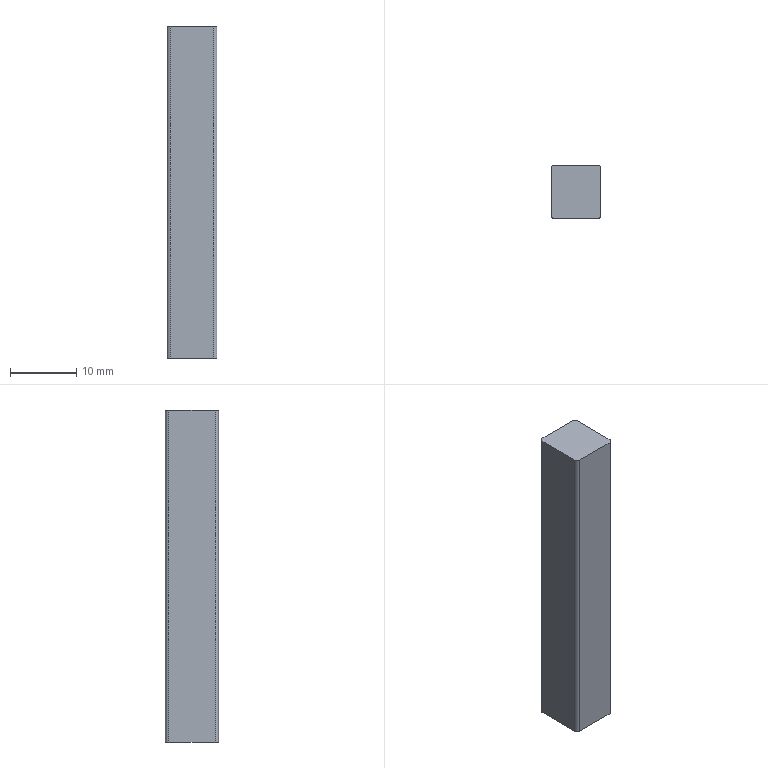Part | NX | features BREP 1 | 1 solid | 10 faces | box 7.5 x 8 x 50 mm | volume 2989 mm3 | plane 6 | cylinder 4 | commonest cylinder face diameters 1 x4
STEP:
#1=CARTESIAN_POINT('',(-3.25,4.,-40.6));
#2=VERTEX_POINT('',#1);
#3=CARTESIAN_POINT('',(-3.75,3.5,-40.6));
#4=VERTEX_POINT('',#3);
#5=CARTESIAN_POINT('',(-3.25,3.5,-40.6));
#6=DIRECTION('',(0.,0.,1.));
#7=DIRECTION('',(1.,0.,0.));
#8=AXIS2_PLACEMENT_3D('',#5,#6,#7);
#9=CIRCLE('',#8,0.5);
#10=EDGE_CURVE('',#2,#4,#9,.T.);
#11=ORIENTED_EDGE('',*,*,#10,.F.);
#12=CARTESIAN_POINT('',(-3.25,4.,-90.6));
#13=VERTEX_POINT('',#12);
#14=CARTESIAN_POINT('',(-3.25,4.,-90.6));
#15=DIRECTION('',(0.,0.,1.));
#16=VECTOR('',#15,1000.);
#17=LINE('',#14,#16);
#18=EDGE_CURVE('',#13,#2,#17,.T.);
#19=ORIENTED_EDGE('',*,*,#18,.F.);
#20=CARTESIAN_POINT('',(-3.75,3.5,-90.6));
#21=VERTEX_POINT('',#20);
#22=CARTESIAN_POINT('',(-3.25,3.5,-90.6));
#23=DIRECTION('',(0.,0.,1.));
#24=DIRECTION('',(1.,0.,0.));
#25=AXIS2_PLACEMENT_3D('',#22,#23,#24);
#26=CIRCLE('',#25,0.5);
#27=EDGE_CURVE('',#13,#21,#26,.T.);
#28=ORIENTED_EDGE('',*,*,#27,.T.);
#29=CARTESIAN_POINT('',(-3.75,3.5,-90.6));
#30=DIRECTION('',(0.,0.,1.));
#31=VECTOR('',#30,1000.);
#32=LINE('',#29,#31);
#33=EDGE_CURVE('',#21,#4,#32,.T.);
#34=ORIENTED_EDGE('',*,*,#33,.T.);
#35=EDGE_LOOP('',(#11,#19,#28,#34));
#36=FACE_BOUND('',#35,.T.);
#37=CARTESIAN_POINT('',(-3.25,3.5,-90.6));
#38=DIRECTION('',(0.,0.,1.));
#39=DIRECTION('',(-1.,0.,0.));
#40=AXIS2_PLACEMENT_3D('',#37,#38,#39);
#41=CYLINDRICAL_SURFACE('',#40,0.5);
#42=ADVANCED_FACE('',(#36),#41,.T.);
#43=CARTESIAN_POINT('',(-3.75,-3.5,-40.6));
#44=VERTEX_POINT('',#43);
#45=CARTESIAN_POINT('',(-3.75,-3.5,-40.6));
#46=DIRECTION('',(0.,1.,0.));
#47=VECTOR('',#46,1000.);
#48=LINE('',#45,#47);
#49=EDGE_CURVE('',#44,#4,#48,.T.);
#50=ORIENTED_EDGE('',*,*,#49,.T.);
#51=ORIENTED_EDGE('',*,*,#33,.F.);
#52=CARTESIAN_POINT('',(-3.75,-3.5,-90.6));
#53=VERTEX_POINT('',#52);
#54=CARTESIAN_POINT('',(-3.75,-3.5,-90.6));
#55=DIRECTION('',(0.,1.,0.));
#56=VECTOR('',#55,1000.);
#57=LINE('',#54,#56);
#58=EDGE_CURVE('',#53,#21,#57,.T.);
#59=ORIENTED_EDGE('',*,*,#58,.F.);
#60=CARTESIAN_POINT('',(-3.75,-3.5,-90.6));
#61=DIRECTION('',(0.,0.,1.));
#62=VECTOR('',#61,1000.);
#63=LINE('',#60,#62);
#64=EDGE_CURVE('',#53,#44,#63,.T.);
#65=ORIENTED_EDGE('',*,*,#64,.T.);
#66=EDGE_LOOP('',(#50,#51,#59,#65));
#67=FACE_BOUND('',#66,.T.);
#68=CARTESIAN_POINT('',(-3.75,-3.5,-90.6));
#69=DIRECTION('',(1.,0.,0.));
#70=DIRECTION('',(0.,0.,1.));
#71=AXIS2_PLACEMENT_3D('',#68,#69,#70);
#72=PLANE('',#71);
#73=ADVANCED_FACE('',(#67),#72,.F.);
#74=CARTESIAN_POINT('',(-3.25,-4.,-40.6));
#75=VERTEX_POINT('',#74);
#76=CARTESIAN_POINT('',(-3.25,-3.5,-40.6));
#77=DIRECTION('',(0.,0.,1.));
#78=DIRECTION('',(1.,0.,0.));
#79=AXIS2_PLACEMENT_3D('',#76,#77,#78);
#80=CIRCLE('',#79,0.5);
#81=EDGE_CURVE('',#44,#75,#80,.T.);
#82=ORIENTED_EDGE('',*,*,#81,.F.);
#83=ORIENTED_EDGE('',*,*,#64,.F.);
#84=CARTESIAN_POINT('',(-3.25,-4.,-90.6));
#85=VERTEX_POINT('',#84);
#86=CARTESIAN_POINT('',(-3.25,-3.5,-90.6));
#87=DIRECTION('',(0.,0.,1.));
#88=DIRECTION('',(1.,0.,0.));
#89=AXIS2_PLACEMENT_3D('',#86,#87,#88);
#90=CIRCLE('',#89,0.5);
#91=EDGE_CURVE('',#53,#85,#90,.T.);
#92=ORIENTED_EDGE('',*,*,#91,.T.);
#93=CARTESIAN_POINT('',(-3.25,-4.,-90.6));
#94=DIRECTION('',(0.,0.,1.));
#95=VECTOR('',#94,1000.);
#96=LINE('',#93,#95);
#97=EDGE_CURVE('',#85,#75,#96,.T.);
#98=ORIENTED_EDGE('',*,*,#97,.T.);
#99=EDGE_LOOP('',(#82,#83,#92,#98));
#100=FACE_BOUND('',#99,.T.);
#101=CARTESIAN_POINT('',(-3.25,-3.5,-90.6));
#102=DIRECTION('',(0.,0.,1.));
#103=DIRECTION('',(-1.,0.,0.));
#104=AXIS2_PLACEMENT_3D('',#101,#102,#103);
#105=CYLINDRICAL_SURFACE('',#104,0.5);
#106=ADVANCED_FACE('',(#100),#105,.T.);
#107=CARTESIAN_POINT('',(3.25,-4.,-40.6));
#108=VERTEX_POINT('',#107);
#109=CARTESIAN_POINT('',(3.25,-4.,-40.6));
#110=DIRECTION('',(-1.,0.,0.));
#111=VECTOR('',#110,1000.);
#112=LINE('',#109,#111);
#113=EDGE_CURVE('',#108,#75,#112,.T.);
#114=ORIENTED_EDGE('',*,*,#113,.T.);
#115=ORIENTED_EDGE('',*,*,#97,.F.);
#116=CARTESIAN_POINT('',(3.25,-4.,-90.6));
#117=VERTEX_POINT('',#116);
#118=CARTESIAN_POINT('',(3.25,-4.,-90.6));
#119=DIRECTION('',(-1.,0.,0.));
#120=VECTOR('',#119,1000.);
#121=LINE('',#118,#120);
#122=EDGE_CURVE('',#117,#85,#121,.T.);
#123=ORIENTED_EDGE('',*,*,#122,.F.);
#124=CARTESIAN_POINT('',(3.25,-4.,-90.6));
#125=DIRECTION('',(0.,0.,1.));
#126=VECTOR('',#125,1000.);
#127=LINE('',#124,#126);
#128=EDGE_CURVE('',#117,#108,#127,.T.);
#129=ORIENTED_EDGE('',*,*,#128,.T.);
#130=EDGE_LOOP('',(#114,#115,#123,#129));
#131=FACE_BOUND('',#130,.T.);
#132=CARTESIAN_POINT('',(3.25,-4.,-90.6));
#133=DIRECTION('',(0.,1.,0.));
#134=DIRECTION('',(0.,0.,-1.));
#135=AXIS2_PLACEMENT_3D('',#132,#133,#134);
#136=PLANE('',#135);
#137=ADVANCED_FACE('',(#131),#136,.F.);
#138=CARTESIAN_POINT('',(3.75,-3.5,-40.6));
#139=VERTEX_POINT('',#138);
#140=CARTESIAN_POINT('',(3.25,-3.5,-40.6));
#141=DIRECTION('',(0.,0.,1.));
#142=DIRECTION('',(1.,0.,0.));
#143=AXIS2_PLACEMENT_3D('',#140,#141,#142);
#144=CIRCLE('',#143,0.5);
#145=EDGE_CURVE('',#108,#139,#144,.T.);
#146=ORIENTED_EDGE('',*,*,#145,.F.);
#147=ORIENTED_EDGE('',*,*,#128,.F.);
#148=CARTESIAN_POINT('',(3.75,-3.5,-90.6));
#149=VERTEX_POINT('',#148);
#150=CARTESIAN_POINT('',(3.25,-3.5,-90.6));
#151=DIRECTION('',(0.,0.,1.));
#152=DIRECTION('',(1.,0.,0.));
#153=AXIS2_PLACEMENT_3D('',#150,#151,#152);
#154=CIRCLE('',#153,0.5);
#155=EDGE_CURVE('',#117,#149,#154,.T.);
#156=ORIENTED_EDGE('',*,*,#155,.T.);
#157=CARTESIAN_POINT('',(3.75,-3.5,-90.6));
#158=DIRECTION('',(0.,0.,1.));
#159=VECTOR('',#158,1000.);
#160=LINE('',#157,#159);
#161=EDGE_CURVE('',#149,#139,#160,.T.);
#162=ORIENTED_EDGE('',*,*,#161,.T.);
#163=EDGE_LOOP('',(#146,#147,#156,#162));
#164=FACE_BOUND('',#163,.T.);
#165=CARTESIAN_POINT('',(3.25,-3.5,-90.6));
#166=DIRECTION('',(0.,0.,1.));
#167=DIRECTION('',(-1.,0.,0.));
#168=AXIS2_PLACEMENT_3D('',#165,#166,#167);
#169=CYLINDRICAL_SURFACE('',#168,0.5);
#170=ADVANCED_FACE('',(#164),#169,.T.);
#171=CARTESIAN_POINT('',(3.75,3.5,-40.6));
#172=VERTEX_POINT('',#171);
#173=CARTESIAN_POINT('',(3.75,3.5,-40.6));
#174=DIRECTION('',(0.,-1.,0.));
#175=VECTOR('',#174,1000.);
#176=LINE('',#173,#175);
#177=EDGE_CURVE('',#172,#139,#176,.T.);
#178=ORIENTED_EDGE('',*,*,#177,.T.);
#179=ORIENTED_EDGE('',*,*,#161,.F.);
#180=CARTESIAN_POINT('',(3.75,3.5,-90.6));
#181=VERTEX_POINT('',#180);
#182=CARTESIAN_POINT('',(3.75,3.5,-90.6));
#183=DIRECTION('',(0.,-1.,0.));
#184=VECTOR('',#183,1000.);
#185=LINE('',#182,#184);
#186=EDGE_CURVE('',#181,#149,#185,.T.);
#187=ORIENTED_EDGE('',*,*,#186,.F.);
#188=CARTESIAN_POINT('',(3.75,3.5,-90.6));
#189=DIRECTION('',(0.,0.,1.));
#190=VECTOR('',#189,1000.);
#191=LINE('',#188,#190);
#192=EDGE_CURVE('',#181,#172,#191,.T.);
#193=ORIENTED_EDGE('',*,*,#192,.T.);
#194=EDGE_LOOP('',(#178,#179,#187,#193));
#195=FACE_BOUND('',#194,.T.);
#196=CARTESIAN_POINT('',(3.75,3.5,-90.6));
#197=DIRECTION('',(-1.,0.,0.));
#198=DIRECTION('',(0.,0.,-1.));
#199=AXIS2_PLACEMENT_3D('',#196,#197,#198);
#200=PLANE('',#199);
#201=ADVANCED_FACE('',(#195),#200,.F.);
#202=CARTESIAN_POINT('',(3.25,4.,-40.6));
#203=VERTEX_POINT('',#202);
#204=CARTESIAN_POINT('',(3.25,3.5,-40.6));
#205=DIRECTION('',(0.,0.,1.));
#206=DIRECTION('',(1.,0.,0.));
#207=AXIS2_PLACEMENT_3D('',#204,#205,#206);
#208=CIRCLE('',#207,0.5);
#209=EDGE_CURVE('',#172,#203,#208,.T.);
#210=ORIENTED_EDGE('',*,*,#209,.F.);
#211=ORIENTED_EDGE('',*,*,#192,.F.);
#212=CARTESIAN_POINT('',(3.25,4.,-90.6));
#213=VERTEX_POINT('',#212);
#214=CARTESIAN_POINT('',(3.25,3.5,-90.6));
#215=DIRECTION('',(0.,0.,1.));
#216=DIRECTION('',(1.,0.,0.));
#217=AXIS2_PLACEMENT_3D('',#214,#215,#216);
#218=CIRCLE('',#217,0.5);
#219=EDGE_CURVE('',#181,#213,#218,.T.);
#220=ORIENTED_EDGE('',*,*,#219,.T.);
#221=CARTESIAN_POINT('',(3.25,4.,-90.6));
#222=DIRECTION('',(0.,0.,1.));
#223=VECTOR('',#222,1000.);
#224=LINE('',#221,#223);
#225=EDGE_CURVE('',#213,#203,#224,.T.);
#226=ORIENTED_EDGE('',*,*,#225,.T.);
#227=EDGE_LOOP('',(#210,#211,#220,#226));
#228=FACE_BOUND('',#227,.T.);
#229=CARTESIAN_POINT('',(3.25,3.5,-90.6));
#230=DIRECTION('',(0.,0.,1.));
#231=DIRECTION('',(-1.,0.,0.));
#232=AXIS2_PLACEMENT_3D('',#229,#230,#231);
#233=CYLINDRICAL_SURFACE('',#232,0.5);
#234=ADVANCED_FACE('',(#228),#233,.T.);
#235=CARTESIAN_POINT('',(-3.25,4.,-40.6));
#236=DIRECTION('',(1.,0.,0.));
#237=VECTOR('',#236,1000.);
#238=LINE('',#235,#237);
#239=EDGE_CURVE('',#2,#203,#238,.T.);
#240=ORIENTED_EDGE('',*,*,#239,.T.);
#241=ORIENTED_EDGE('',*,*,#225,.F.);
#242=CARTESIAN_POINT('',(-3.25,4.,-90.6));
#243=DIRECTION('',(1.,0.,0.));
#244=VECTOR('',#243,1000.);
#245=LINE('',#242,#244);
#246=EDGE_CURVE('',#13,#213,#245,.T.);
#247=ORIENTED_EDGE('',*,*,#246,.F.);
#248=ORIENTED_EDGE('',*,*,#18,.T.);
#249=EDGE_LOOP('',(#240,#241,#247,#248));
#250=FACE_BOUND('',#249,.T.);
#251=CARTESIAN_POINT('',(-3.25,4.,-90.6));
#252=DIRECTION('',(0.,-1.,0.));
#253=DIRECTION('',(0.,0.,1.));
#254=AXIS2_PLACEMENT_3D('',#251,#252,#253);
#255=PLANE('',#254);
#256=ADVANCED_FACE('',(#250),#255,.F.);
#257=ORIENTED_EDGE('',*,*,#27,.F.);
#258=ORIENTED_EDGE('',*,*,#246,.T.);
#259=ORIENTED_EDGE('',*,*,#219,.F.);
#260=ORIENTED_EDGE('',*,*,#186,.T.);
#261=ORIENTED_EDGE('',*,*,#155,.F.);
#262=ORIENTED_EDGE('',*,*,#122,.T.);
#263=ORIENTED_EDGE('',*,*,#91,.F.);
#264=ORIENTED_EDGE('',*,*,#58,.T.);
#265=EDGE_LOOP('',(#257,#258,#259,#260,#261,#262,#263,#264));
#266=FACE_BOUND('',#265,.T.);
#267=CARTESIAN_POINT('',(-3.25,3.5,-90.6));
#268=DIRECTION('',(0.,0.,1.));
#269=DIRECTION('',(-1.,0.,0.));
#270=AXIS2_PLACEMENT_3D('',#267,#268,#269);
#271=PLANE('',#270);
#272=ADVANCED_FACE('',(#266),#271,.F.);
#273=ORIENTED_EDGE('',*,*,#10,.T.);
#274=ORIENTED_EDGE('',*,*,#49,.F.);
#275=ORIENTED_EDGE('',*,*,#81,.T.);
#276=ORIENTED_EDGE('',*,*,#113,.F.);
#277=ORIENTED_EDGE('',*,*,#145,.T.);
#278=ORIENTED_EDGE('',*,*,#177,.F.);
#279=ORIENTED_EDGE('',*,*,#209,.T.);
#280=ORIENTED_EDGE('',*,*,#239,.F.);
#281=EDGE_LOOP('',(#273,#274,#275,#276,#277,#278,#279,#280));
#282=FACE_BOUND('',#281,.T.);
#283=CARTESIAN_POINT('',(-3.25,3.5,-40.6));
#284=DIRECTION('',(0.,0.,1.));
#285=DIRECTION('',(-1.,0.,0.));
#286=AXIS2_PLACEMENT_3D('',#283,#284,#285);
#287=PLANE('',#286);
#288=ADVANCED_FACE('',(#282),#287,.T.);
#289=CLOSED_SHELL('',(#42,#73,#106,#137,#170,#201,#234,#256,#272,#288));
#290=MANIFOLD_SOLID_BREP('',#289);
#291=(LENGTH_UNIT()NAMED_UNIT(*)SI_UNIT(.MILLI.,.METRE.));
#292=UNCERTAINTY_MEASURE_WITH_UNIT(LENGTH_MEASURE(0.00001),#291,'','');
#293=(NAMED_UNIT(*)PLANE_ANGLE_UNIT()SI_UNIT($,.RADIAN.));
#294=(NAMED_UNIT(*)SI_UNIT($,.STERADIAN.)SOLID_ANGLE_UNIT());
#295=(GEOMETRIC_REPRESENTATION_CONTEXT(3)GLOBAL_UNCERTAINTY_ASSIGNED_CONTEXT((#292))GLOBAL_UNIT_ASSIGNED_CONTEXT((#291,#293,#294))REPRESENTATION_CONTEXT('',''));
#296=ADVANCED_BREP_SHAPE_REPRESENTATION('',(#290),#295);